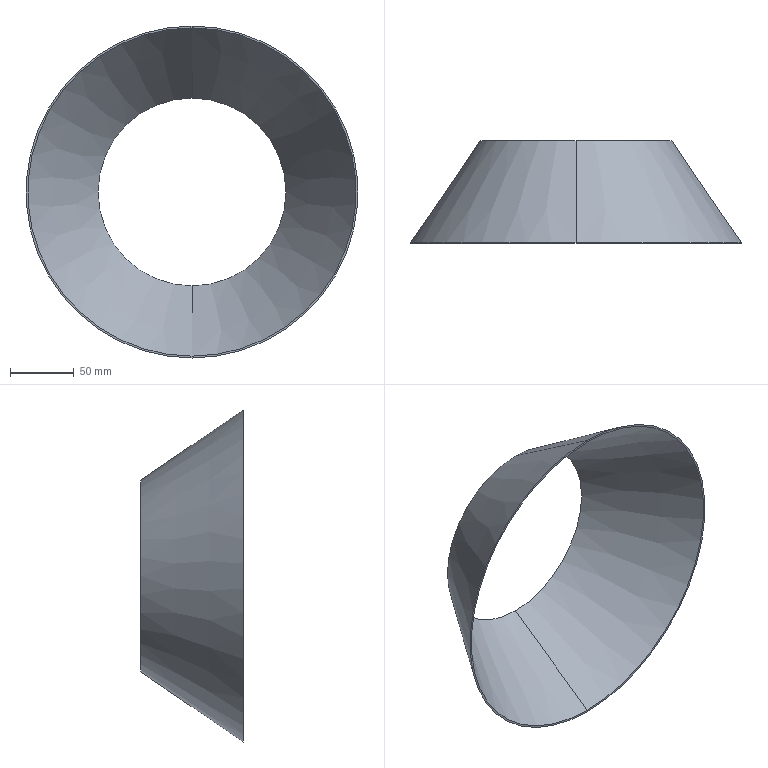Part | SolidWorks | features Revolution 1, Shell 1 | 1 solid | 6 faces | box 260 x 80 x 260 mm | volume 74495 mm3 | cone 4 | plane 2
STEP:
#1=CARTESIAN_POINT('',(0.,80.,73.544));
#2=VERTEX_POINT('',#1);
#3=CARTESIAN_POINT('',(0.,80.,-73.544));
#4=VERTEX_POINT('',#3);
#5=CARTESIAN_POINT('',(0.,80.,0.));
#6=DIRECTION('',(0.,-1.,0.));
#7=DIRECTION('',(0.,0.,1.));
#8=AXIS2_PLACEMENT_3D('',#5,#6,#7);
#9=CIRCLE('',#8,73.544);
#10=EDGE_CURVE('',#2,#4,#9,.T.);
#11=ORIENTED_EDGE('',*,*,#10,.F.);
#12=CARTESIAN_POINT('',(0.,0.,128.544));
#13=VERTEX_POINT('',#12);
#14=CARTESIAN_POINT('',(0.,-0.6798,129.011));
#15=DIRECTION('',(0.,-0.824,0.5665));
#16=VECTOR('',#15,1000.);
#17=LINE('',#14,#16);
#18=EDGE_CURVE('',#2,#13,#17,.T.);
#19=ORIENTED_EDGE('',*,*,#18,.T.);
#20=CARTESIAN_POINT('',(0.,0.,-128.544));
#21=VERTEX_POINT('',#20);
#22=CARTESIAN_POINT('',(0.,0.,0.));
#23=DIRECTION('',(0.,-1.,0.));
#24=DIRECTION('',(0.,0.,-1.));
#25=AXIS2_PLACEMENT_3D('',#22,#23,#24);
#26=CIRCLE('',#25,128.544);
#27=EDGE_CURVE('',#13,#21,#26,.T.);
#28=ORIENTED_EDGE('',*,*,#27,.T.);
#29=CARTESIAN_POINT('',(0.,-0.6798,-129.011));
#30=DIRECTION('',(0.,-0.824,-0.5665));
#31=VECTOR('',#30,1000.);
#32=LINE('',#29,#31);
#33=EDGE_CURVE('',#4,#21,#32,.T.);
#34=ORIENTED_EDGE('',*,*,#33,.F.);
#35=EDGE_LOOP('',(#11,#19,#28,#34));
#36=FACE_OUTER_BOUND('',#35,.T.);
#37=CARTESIAN_POINT('',(0.,-0.6798,0.));
#38=DIRECTION('',(0.,-1.,0.));
#39=DIRECTION('',(0.,0.,-1.));
#40=AXIS2_PLACEMENT_3D('',#37,#38,#39);
#41=CONICAL_SURFACE('',#40,129.011,0.6023);
#42=ADVANCED_FACE('',(#36),#41,.F.);
#43=CARTESIAN_POINT('',(0.,80.,-75.));
#44=VERTEX_POINT('',#43);
#45=CARTESIAN_POINT('',(0.,80.,75.));
#46=VERTEX_POINT('',#45);
#47=CARTESIAN_POINT('',(0.,80.,0.));
#48=DIRECTION('',(0.,-1.,0.));
#49=DIRECTION('',(0.,0.,-1.));
#50=AXIS2_PLACEMENT_3D('',#47,#48,#49);
#51=CIRCLE('',#50,75.);
#52=EDGE_CURVE('',#44,#46,#51,.T.);
#53=ORIENTED_EDGE('',*,*,#52,.T.);
#54=CARTESIAN_POINT('',(0.,0.,130.));
#55=VERTEX_POINT('',#54);
#56=CARTESIAN_POINT('',(0.,0.,130.));
#57=DIRECTION('',(0.,-0.824,0.5665));
#58=VECTOR('',#57,1000.);
#59=LINE('',#56,#58);
#60=EDGE_CURVE('',#46,#55,#59,.T.);
#61=ORIENTED_EDGE('',*,*,#60,.T.);
#62=CARTESIAN_POINT('',(0.,0.,-130.));
#63=VERTEX_POINT('',#62);
#64=CARTESIAN_POINT('',(0.,0.,0.));
#65=DIRECTION('',(0.,-1.,0.));
#66=DIRECTION('',(0.,0.,-1.));
#67=AXIS2_PLACEMENT_3D('',#64,#65,#66);
#68=CIRCLE('',#67,130.);
#69=EDGE_CURVE('',#63,#55,#68,.T.);
#70=ORIENTED_EDGE('',*,*,#69,.F.);
#71=CARTESIAN_POINT('',(0.,0.,-130.));
#72=DIRECTION('',(0.,-0.824,-0.5665));
#73=VECTOR('',#72,1000.);
#74=LINE('',#71,#73);
#75=EDGE_CURVE('',#44,#63,#74,.T.);
#76=ORIENTED_EDGE('',*,*,#75,.F.);
#77=EDGE_LOOP('',(#53,#61,#70,#76));
#78=FACE_OUTER_BOUND('',#77,.T.);
#79=CARTESIAN_POINT('',(0.,0.,0.));
#80=DIRECTION('',(0.,-1.,0.));
#81=DIRECTION('',(0.,0.,-1.));
#82=AXIS2_PLACEMENT_3D('',#79,#80,#81);
#83=CONICAL_SURFACE('',#82,130.,0.6023);
#84=ADVANCED_FACE('',(#78),#83,.T.);
#85=CARTESIAN_POINT('',(0.,80.,0.));
#86=DIRECTION('',(0.,-1.,0.));
#87=DIRECTION('',(0.,0.,1.));
#88=AXIS2_PLACEMENT_3D('',#85,#86,#87);
#89=CIRCLE('',#88,73.544);
#90=EDGE_CURVE('',#4,#2,#89,.T.);
#91=ORIENTED_EDGE('',*,*,#90,.T.);
#92=ORIENTED_EDGE('',*,*,#10,.T.);
#93=EDGE_LOOP('',(#91,#92));
#94=FACE_BOUND('',#93,.T.);
#95=ORIENTED_EDGE('',*,*,#52,.F.);
#96=CARTESIAN_POINT('',(0.,80.,0.));
#97=DIRECTION('',(0.,-1.,0.));
#98=DIRECTION('',(0.,0.,-1.));
#99=AXIS2_PLACEMENT_3D('',#96,#97,#98);
#100=CIRCLE('',#99,75.);
#101=EDGE_CURVE('',#46,#44,#100,.T.);
#102=ORIENTED_EDGE('',*,*,#101,.F.);
#103=EDGE_LOOP('',(#95,#102));
#104=FACE_OUTER_BOUND('',#103,.T.);
#105=CARTESIAN_POINT('',(0.,80.,0.));
#106=DIRECTION('',(0.,1.,0.));
#107=DIRECTION('',(0.,0.,1.));
#108=AXIS2_PLACEMENT_3D('',#105,#106,#107);
#109=PLANE('',#108);
#110=ADVANCED_FACE('',(#94,#104),#109,.T.);
#111=ORIENTED_EDGE('',*,*,#60,.F.);
#112=ORIENTED_EDGE('',*,*,#101,.T.);
#113=ORIENTED_EDGE('',*,*,#75,.T.);
#114=CARTESIAN_POINT('',(0.,0.,0.));
#115=DIRECTION('',(0.,-1.,0.));
#116=DIRECTION('',(0.,0.,-1.));
#117=AXIS2_PLACEMENT_3D('',#114,#115,#116);
#118=CIRCLE('',#117,130.);
#119=EDGE_CURVE('',#55,#63,#118,.T.);
#120=ORIENTED_EDGE('',*,*,#119,.F.);
#121=EDGE_LOOP('',(#111,#112,#113,#120));
#122=FACE_OUTER_BOUND('',#121,.T.);
#123=CARTESIAN_POINT('',(0.,0.,0.));
#124=DIRECTION('',(0.,-1.,0.));
#125=DIRECTION('',(0.,0.,-1.));
#126=AXIS2_PLACEMENT_3D('',#123,#124,#125);
#127=CONICAL_SURFACE('',#126,130.,0.6023);
#128=ADVANCED_FACE('',(#122),#127,.T.);
#129=CARTESIAN_POINT('',(0.,0.,0.));
#130=DIRECTION('',(0.,-1.,0.));
#131=DIRECTION('',(0.,0.,-1.));
#132=AXIS2_PLACEMENT_3D('',#129,#130,#131);
#133=CIRCLE('',#132,128.544);
#134=EDGE_CURVE('',#21,#13,#133,.T.);
#135=ORIENTED_EDGE('',*,*,#134,.F.);
#136=ORIENTED_EDGE('',*,*,#27,.F.);
#137=EDGE_LOOP('',(#135,#136));
#138=FACE_BOUND('',#137,.T.);
#139=ORIENTED_EDGE('',*,*,#69,.T.);
#140=ORIENTED_EDGE('',*,*,#119,.T.);
#141=EDGE_LOOP('',(#139,#140));
#142=FACE_OUTER_BOUND('',#141,.T.);
#143=CARTESIAN_POINT('',(130.,0.,0.));
#144=DIRECTION('',(0.,-1.,0.));
#145=DIRECTION('',(0.,0.,-1.));
#146=AXIS2_PLACEMENT_3D('',#143,#144,#145);
#147=PLANE('',#146);
#148=ADVANCED_FACE('',(#138,#142),#147,.T.);
#149=ORIENTED_EDGE('',*,*,#18,.F.);
#150=ORIENTED_EDGE('',*,*,#90,.F.);
#151=ORIENTED_EDGE('',*,*,#33,.T.);
#152=ORIENTED_EDGE('',*,*,#134,.T.);
#153=EDGE_LOOP('',(#149,#150,#151,#152));
#154=FACE_OUTER_BOUND('',#153,.T.);
#155=CARTESIAN_POINT('',(0.,-0.6798,0.));
#156=DIRECTION('',(0.,-1.,0.));
#157=DIRECTION('',(0.,0.,-1.));
#158=AXIS2_PLACEMENT_3D('',#155,#156,#157);
#159=CONICAL_SURFACE('',#158,129.011,0.6023);
#160=ADVANCED_FACE('',(#154),#159,.F.);
#161=CLOSED_SHELL('',(#42,#84,#110,#128,#148,#160));
#162=MANIFOLD_SOLID_BREP('',#161);
#163=CARTESIAN_POINT('',(0.,0.,0.));
#164=DIRECTION('',(0.,0.,1.));
#165=DIRECTION('',(1.,0.,0.));
#166=AXIS2_PLACEMENT_3D('',#163,#164,#165);
#167=(LENGTH_UNIT()NAMED_UNIT(*)SI_UNIT(.MILLI.,.METRE.));
#168=UNCERTAINTY_MEASURE_WITH_UNIT(LENGTH_MEASURE(0.00001),#167,'','');
#169=(NAMED_UNIT(*)PLANE_ANGLE_UNIT()SI_UNIT($,.RADIAN.));
#170=(NAMED_UNIT(*)SI_UNIT($,.STERADIAN.)SOLID_ANGLE_UNIT());
#171=(GEOMETRIC_REPRESENTATION_CONTEXT(3)GLOBAL_UNCERTAINTY_ASSIGNED_CONTEXT((#168))GLOBAL_UNIT_ASSIGNED_CONTEXT((#167,#169,#170))REPRESENTATION_CONTEXT('',''));
#172=ADVANCED_BREP_SHAPE_REPRESENTATION('',(#162,#166),#171);